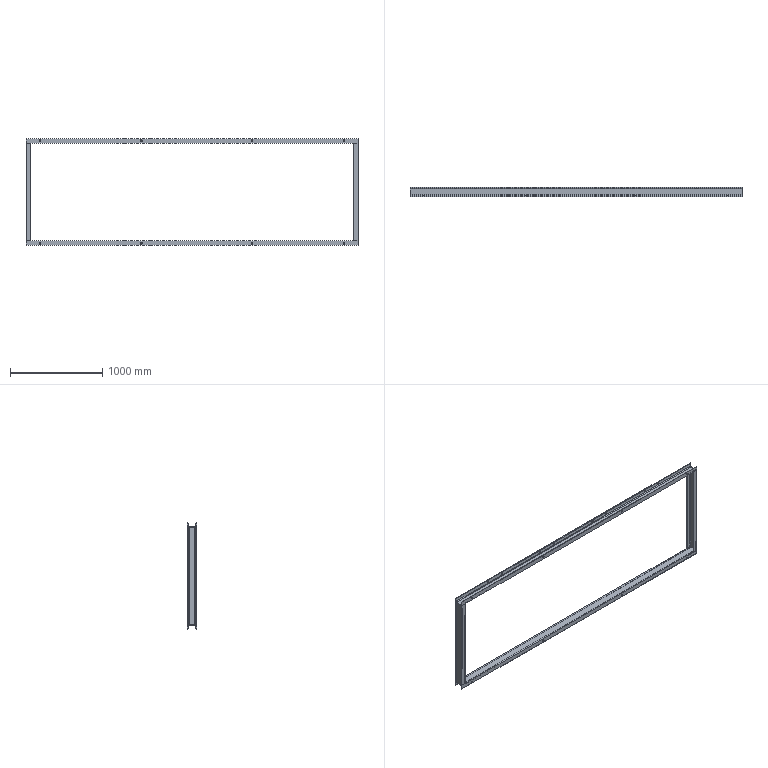Part | STEP file | SW-102-Base2_default<by machining> | 4 solids | 104 faces | box 3604 x 100 x 1155 mm | volume 11682960 mm3 | cylinder 64 | plane 40 | commonest cylinder face diameters 18 x48 8.5 x8 17 x8